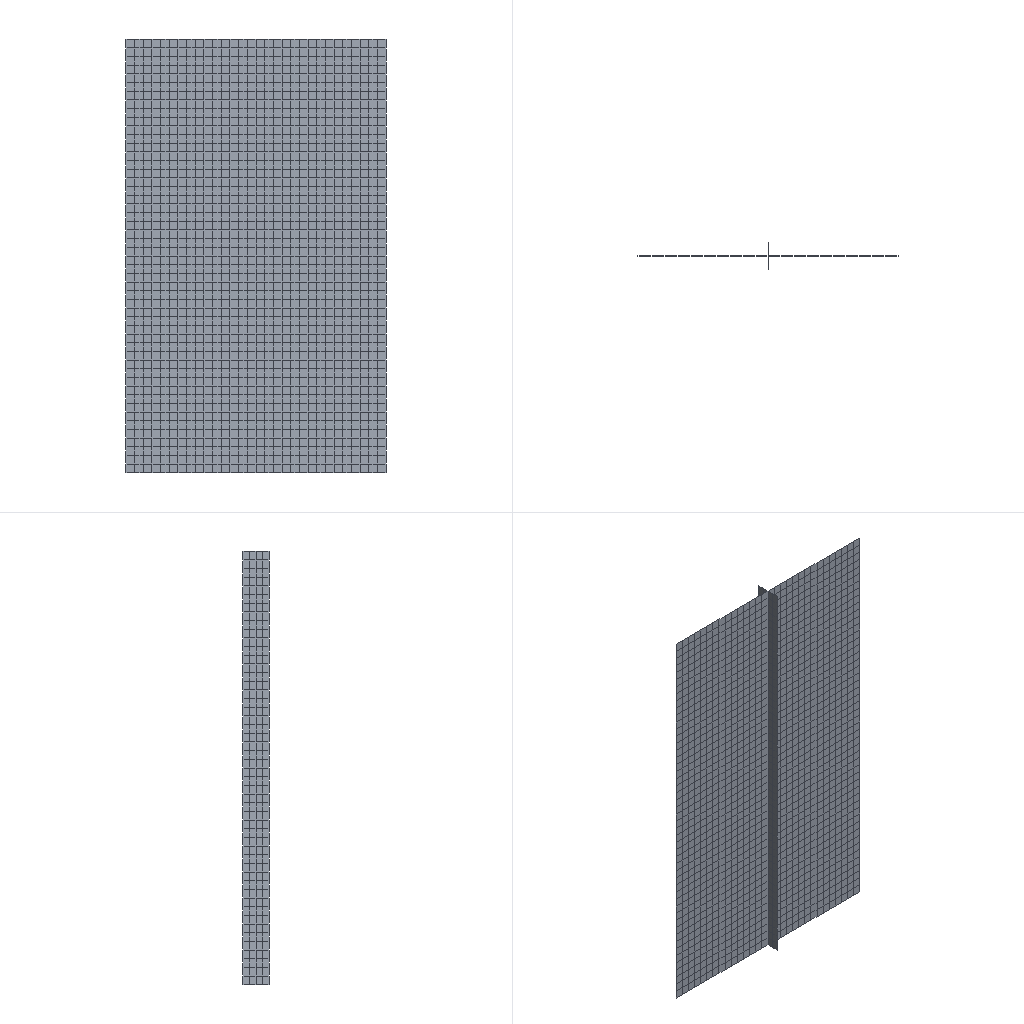Simulation study | abaqus
Set-up summary:
category,name,step,type,value,unit,region
solver,abaqus
solver,version,,,Abaqus/Standard 6.13-1
units,not stated in the deck,,not stated
analysis,deck,,buckling,buckling
load_step,Step-1,Step-1,buckling
load_step,requested,,,1
mesh,nodes,,,1785
mesh,elements,,,1700
element_type,S4R,,shell,1700
load,load commands in deck,,count,1
bc,support commands in deck,,count,4
material,MATERIAL-1,,in results
check,setup vs results,,match,"per instance, exact: element labels, types and connectivity; labels of the nodes the elements use; coordinates of those nodes at SINGLE_PRECISION in 1 of 1 instance(s)"
Abaqus input file, long lists of numbers shortened:
*Heading
** Job name:  Model name: Model-1
** Generated by: Abaqus/CAE 6.13-1
*Preprint, echo=NO, model=NO, history=NO, contact=NO
**
** PARTS
**
*Part, name=Part-1
*Node
      1,           0.,           0.,           0.
      2,           0.,           0.,         100.
** (1783 more lines like these left out)
*Element, type=S4R
  1,    1,   11,  316,  136
  2,   11,   12,  317,  316
** (1698 more lines like these left out)
*Nset, nset=_PickedSet2, internal, generate
    1,  1785,     1
*Elset, elset=_PickedSet2, internal, generate
    1,  1700,     1
** Section: Section-1
*Shell Section, elset=_PickedSet2, material=Material-1
0.5, 5
*End Part
**
**
** ASSEMBLY
**
*Assembly, name=Assembly
**
*Instance, name=Part-1-1, part=Part-1
*End Instance
**
*Nset, nset=_PickedSet5, internal, instance=Part-1-1
   1,   4,   5,   8,   9, 123, 124, 125, 126, 127, 128, 129, 130, 131, 132, 133
 134, 135, 136, 137, 138, 139, 140, 141, 142, 143, 144, 145, 146, 147, 148, 149
** (1 more lines like these left out)
*Elset, elset=_PickedSet5, internal, instance=Part-1-1
    1,   51,  101,  151,  201,  251,  301,  351,  401,  451,  501,  551,  601,  651,  701,  800
  850,  900,  950, 1000, 1050, 1100, 1150, 1200, 1250, 1300, 1350, 1400, 1450, 1500, 1501, 1551
** (1 more lines like these left out)
*Nset, nset=_PickedSet6, internal, instance=Part-1-1
   2,   3,   4,   5,   6,  60,  61,  62,  63,  64,  65,  66,  67,  68,  69,  70
  71,  72,  73,  74,  75,  76,  77,  78,  79,  80,  81,  82,  83,  84,  85,  86
** (7 more lines like these left out)
*Elset, elset=_PickedSet6, internal, instance=Part-1-1
   50,  100,  150,  200,  250,  300,  350,  400,  450,  500,  550,  600,  650,  700,  701,  702
  703,  704,  705,  706,  707,  708,  709,  710,  711,  712,  713,  714,  715,  716,  717,  718
** (6 more lines like these left out)
*Elset, elset=__PickedSurf4_E2, internal, instance=Part-1-1
   50,  100,  150,  200,  250,  300,  350,  400,  450,  500,  550,  600,  650,  700,  750, 1550
 1600,
*Elset, elset=__PickedSurf4_E4, internal, instance=Part-1-1
  751,  801,  851,  901,  951, 1001, 1051, 1101, 1151, 1201, 1251, 1301, 1351, 1401, 1451, 1601
 1651,
*Surface, type=ELEMENT, name=_PickedSurf4, internal
__PickedSurf4_E2, E2
__PickedSurf4_E4, E4
*End Assembly
**
** MATERIALS
**
*Material, name=Material-1
*Elastic
19700., 0.3
*Plastic
520.,  0.
950., 0.1
** ----------------------------------------------------------------
**
** STEP: Step-1
**
*Step, name=Step-1, nlgeom=NO, perturbation
*Buckle
6, , 12, 30
**
** BOUNDARY CONDITIONS
**
** Name: BC-1 Type: Symmetry/Antisymmetry/Encastre
*Boundary, op=NEW, load case=1
_PickedSet5, ENCASTRE
*Boundary, op=NEW, load case=2
_PickedSet5, ENCASTRE
** Name: BC-2 Type: Displacement/Rotation
*Boundary, op=NEW, load case=1
_PickedSet6, 2, 2
*Boundary, op=NEW, load case=2
_PickedSet6, 2, 2
**
** LOADS
**
** Name: Load-1   Type: Shell edge load
*Dsload
_PickedSurf4, EDNOR, 1.
**
** OUTPUT REQUESTS
**
*Restart, write, frequency=0
**
** FIELD OUTPUT: F-Output-1
**
*Output, field, variable=PRESELECT
*NODE FILE, GLOBAL=YES, LAST MODE=1
U
*End Step
Results summary:
result,step,Step-1,partial,increments=0 time=0.0/1e-36
result,analysis,,,buckling
result,last_loadstep,,,1
result,primary field,,,"U, UR"